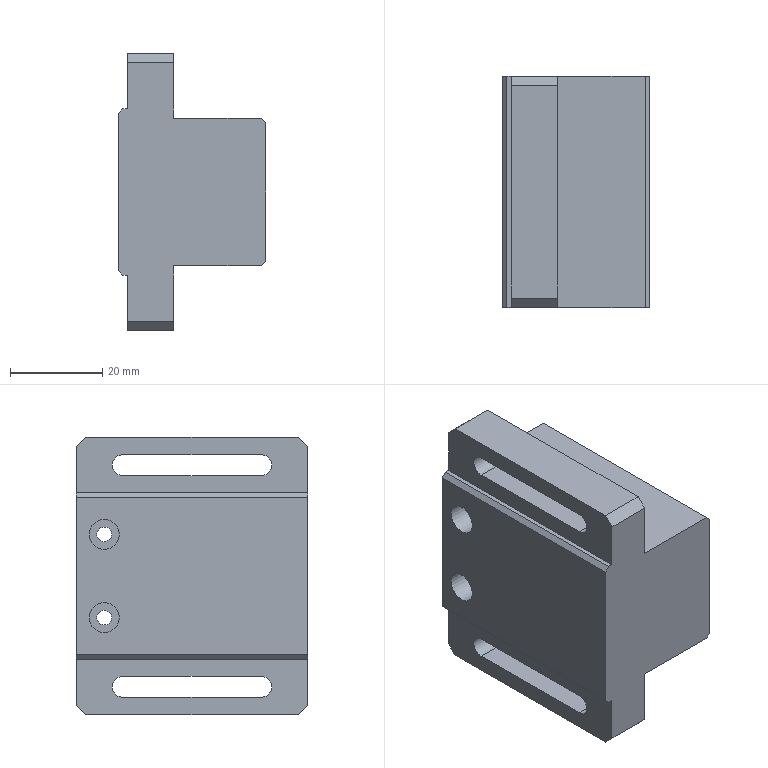Part | NX | 1 solid | 36 faces | box 32 x 50 x 60 mm | volume 61384 mm3 | plane 28 | cylinder 8 | commonest cylinder face diameters 4.5 x4 3.2 x2 6.5 x2
STEP:
#1=CARTESIAN_POINT('',(-15.,23.,-30.));
#2=VERTEX_POINT('',#1);
#3=CARTESIAN_POINT('',(-15.,-23.,-30.));
#4=VERTEX_POINT('',#3);
#5=CARTESIAN_POINT('',(-15.,25.,-30.));
#6=DIRECTION('',(0.,-1.,0.));
#7=VECTOR('',#6,1000.);
#8=LINE('',#5,#7);
#9=EDGE_CURVE('',#2,#4,#8,.T.);
#10=ORIENTED_EDGE('',*,*,#9,.F.);
#11=CARTESIAN_POINT('',(-5.,23.,-30.));
#12=VERTEX_POINT('',#11);
#13=CARTESIAN_POINT('',(-5.,23.,-30.));
#14=DIRECTION('',(1.,0.,0.));
#15=VECTOR('',#14,1000.);
#16=LINE('',#13,#15);
#17=EDGE_CURVE('',#2,#12,#16,.T.);
#18=ORIENTED_EDGE('',*,*,#17,.T.);
#19=CARTESIAN_POINT('',(-5.,-23.,-30.));
#20=VERTEX_POINT('',#19);
#21=CARTESIAN_POINT('',(-5.,25.,-30.));
#22=DIRECTION('',(0.,1.,0.));
#23=VECTOR('',#22,1000.);
#24=LINE('',#21,#23);
#25=EDGE_CURVE('',#20,#12,#24,.T.);
#26=ORIENTED_EDGE('',*,*,#25,.F.);
#27=CARTESIAN_POINT('',(-15.,-23.,-30.));
#28=DIRECTION('',(-1.,0.,0.));
#29=VECTOR('',#28,1000.);
#30=LINE('',#27,#29);
#31=EDGE_CURVE('',#20,#4,#30,.T.);
#32=ORIENTED_EDGE('',*,*,#31,.T.);
#33=EDGE_LOOP('',(#10,#18,#26,#32));
#34=FACE_BOUND('',#33,.T.);
#35=CARTESIAN_POINT('',(-15.,25.,-30.));
#36=DIRECTION('',(0.,0.,1.));
#37=DIRECTION('',(1.,0.,0.));
#38=AXIS2_PLACEMENT_3D('',#35,#36,#37);
#39=PLANE('',#38);
#40=ADVANCED_FACE('',(#34),#39,.F.);
#41=CARTESIAN_POINT('',(-15.,23.,30.));
#42=VERTEX_POINT('',#41);
#43=CARTESIAN_POINT('',(-15.,-23.,30.));
#44=VERTEX_POINT('',#43);
#45=CARTESIAN_POINT('',(-15.,25.,30.));
#46=DIRECTION('',(0.,-1.,0.));
#47=VECTOR('',#46,1000.);
#48=LINE('',#45,#47);
#49=EDGE_CURVE('',#42,#44,#48,.T.);
#50=ORIENTED_EDGE('',*,*,#49,.T.);
#51=CARTESIAN_POINT('',(-5.,-23.,30.));
#52=VERTEX_POINT('',#51);
#53=CARTESIAN_POINT('',(-15.,-23.,30.));
#54=DIRECTION('',(1.,0.,0.));
#55=VECTOR('',#54,1000.);
#56=LINE('',#53,#55);
#57=EDGE_CURVE('',#44,#52,#56,.T.);
#58=ORIENTED_EDGE('',*,*,#57,.T.);
#59=CARTESIAN_POINT('',(-5.,23.,30.));
#60=VERTEX_POINT('',#59);
#61=CARTESIAN_POINT('',(-5.,25.,30.));
#62=DIRECTION('',(0.,-1.,0.));
#63=VECTOR('',#62,1000.);
#64=LINE('',#61,#63);
#65=EDGE_CURVE('',#60,#52,#64,.T.);
#66=ORIENTED_EDGE('',*,*,#65,.F.);
#67=CARTESIAN_POINT('',(-15.,23.,30.));
#68=DIRECTION('',(-1.,0.,0.));
#69=VECTOR('',#68,1000.);
#70=LINE('',#67,#69);
#71=EDGE_CURVE('',#60,#42,#70,.T.);
#72=ORIENTED_EDGE('',*,*,#71,.T.);
#73=EDGE_LOOP('',(#50,#58,#66,#72));
#74=FACE_BOUND('',#73,.T.);
#75=CARTESIAN_POINT('',(-15.,25.,30.));
#76=DIRECTION('',(0.,0.,-1.));
#77=DIRECTION('',(-1.,0.,0.));
#78=AXIS2_PLACEMENT_3D('',#75,#76,#77);
#79=PLANE('',#78);
#80=ADVANCED_FACE('',(#74),#79,.F.);
#81=CARTESIAN_POINT('',(-5.,15.,-21.75));
#82=VERTEX_POINT('',#81);
#83=CARTESIAN_POINT('',(-5.,15.,-26.25));
#84=VERTEX_POINT('',#83);
#85=CARTESIAN_POINT('',(-5.,15.,-24.));
#86=DIRECTION('',(1.,0.,0.));
#87=DIRECTION('',(0.,0.,-1.));
#88=AXIS2_PLACEMENT_3D('',#85,#86,#87);
#89=CIRCLE('',#88,2.25);
#90=EDGE_CURVE('',#82,#84,#89,.F.);
#91=ORIENTED_EDGE('',*,*,#90,.F.);
#92=CARTESIAN_POINT('',(-15.,15.,-21.75));
#93=VERTEX_POINT('',#92);
#94=CARTESIAN_POINT('',(-17.,15.,-21.75));
#95=DIRECTION('',(1.,0.,0.));
#96=VECTOR('',#95,1000.);
#97=LINE('',#94,#96);
#98=EDGE_CURVE('',#93,#82,#97,.T.);
#99=ORIENTED_EDGE('',*,*,#98,.F.);
#100=CARTESIAN_POINT('',(-15.,15.,-26.25));
#101=VERTEX_POINT('',#100);
#102=CARTESIAN_POINT('',(-15.,15.,-24.));
#103=DIRECTION('',(1.,0.,0.));
#104=DIRECTION('',(0.,0.,-1.));
#105=AXIS2_PLACEMENT_3D('',#102,#103,#104);
#106=CIRCLE('',#105,2.25);
#107=EDGE_CURVE('',#101,#93,#106,.T.);
#108=ORIENTED_EDGE('',*,*,#107,.F.);
#109=CARTESIAN_POINT('',(-17.,15.,-26.25));
#110=DIRECTION('',(1.,0.,0.));
#111=VECTOR('',#110,1000.);
#112=LINE('',#109,#111);
#113=EDGE_CURVE('',#101,#84,#112,.T.);
#114=ORIENTED_EDGE('',*,*,#113,.T.);
#115=EDGE_LOOP('',(#91,#99,#108,#114));
#116=FACE_BOUND('',#115,.T.);
#117=CARTESIAN_POINT('',(-17.,15.,-24.));
#118=DIRECTION('',(1.,0.,0.));
#119=DIRECTION('',(0.,0.,-1.));
#120=AXIS2_PLACEMENT_3D('',#117,#118,#119);
#121=CYLINDRICAL_SURFACE('',#120,2.25);
#122=ADVANCED_FACE('',(#116),#121,.F.);
#123=CARTESIAN_POINT('',(-5.,-15.,-26.25));
#124=VERTEX_POINT('',#123);
#125=CARTESIAN_POINT('',(-5.,15.,-26.25));
#126=DIRECTION('',(0.,-1.,0.));
#127=VECTOR('',#126,1000.);
#128=LINE('',#125,#127);
#129=EDGE_CURVE('',#84,#124,#128,.T.);
#130=ORIENTED_EDGE('',*,*,#129,.F.);
#131=ORIENTED_EDGE('',*,*,#113,.F.);
#132=CARTESIAN_POINT('',(-15.,-15.,-26.25));
#133=VERTEX_POINT('',#132);
#134=CARTESIAN_POINT('',(-15.,25.,-26.25));
#135=DIRECTION('',(0.,1.,0.));
#136=VECTOR('',#135,1000.);
#137=LINE('',#134,#136);
#138=EDGE_CURVE('',#133,#101,#137,.T.);
#139=ORIENTED_EDGE('',*,*,#138,.F.);
#140=CARTESIAN_POINT('',(-17.,-15.,-26.25));
#141=DIRECTION('',(1.,0.,0.));
#142=VECTOR('',#141,1000.);
#143=LINE('',#140,#142);
#144=EDGE_CURVE('',#133,#124,#143,.T.);
#145=ORIENTED_EDGE('',*,*,#144,.T.);
#146=EDGE_LOOP('',(#130,#131,#139,#145));
#147=FACE_BOUND('',#146,.T.);
#148=CARTESIAN_POINT('',(-17.,15.,-26.25));
#149=DIRECTION('',(0.,0.,-1.));
#150=DIRECTION('',(-1.,0.,0.));
#151=AXIS2_PLACEMENT_3D('',#148,#149,#150);
#152=PLANE('',#151);
#153=ADVANCED_FACE('',(#147),#152,.F.);
#154=CARTESIAN_POINT('',(-5.,-15.,-21.75));
#155=VERTEX_POINT('',#154);
#156=CARTESIAN_POINT('',(-5.,-15.,-24.));
#157=DIRECTION('',(1.,0.,0.));
#158=DIRECTION('',(0.,0.,-1.));
#159=AXIS2_PLACEMENT_3D('',#156,#157,#158);
#160=CIRCLE('',#159,2.25);
#161=EDGE_CURVE('',#124,#155,#160,.F.);
#162=ORIENTED_EDGE('',*,*,#161,.F.);
#163=ORIENTED_EDGE('',*,*,#144,.F.);
#164=CARTESIAN_POINT('',(-15.,-15.,-21.75));
#165=VERTEX_POINT('',#164);
#166=CARTESIAN_POINT('',(-15.,-15.,-24.));
#167=DIRECTION('',(1.,0.,0.));
#168=DIRECTION('',(0.,0.,-1.));
#169=AXIS2_PLACEMENT_3D('',#166,#167,#168);
#170=CIRCLE('',#169,2.25);
#171=EDGE_CURVE('',#165,#133,#170,.T.);
#172=ORIENTED_EDGE('',*,*,#171,.F.);
#173=CARTESIAN_POINT('',(-17.,-15.,-21.75));
#174=DIRECTION('',(1.,0.,0.));
#175=VECTOR('',#174,1000.);
#176=LINE('',#173,#175);
#177=EDGE_CURVE('',#165,#155,#176,.T.);
#178=ORIENTED_EDGE('',*,*,#177,.T.);
#179=EDGE_LOOP('',(#162,#163,#172,#178));
#180=FACE_BOUND('',#179,.T.);
#181=CARTESIAN_POINT('',(-17.,-15.,-24.));
#182=DIRECTION('',(1.,0.,0.));
#183=DIRECTION('',(0.,0.,-1.));
#184=AXIS2_PLACEMENT_3D('',#181,#182,#183);
#185=CYLINDRICAL_SURFACE('',#184,2.25);
#186=ADVANCED_FACE('',(#180),#185,.F.);
#187=CARTESIAN_POINT('',(-5.,15.,-21.75));
#188=DIRECTION('',(0.,1.,0.));
#189=VECTOR('',#188,1000.);
#190=LINE('',#187,#189);
#191=EDGE_CURVE('',#155,#82,#190,.T.);
#192=ORIENTED_EDGE('',*,*,#191,.F.);
#193=ORIENTED_EDGE('',*,*,#177,.F.);
#194=CARTESIAN_POINT('',(-15.,25.,-21.75));
#195=DIRECTION('',(0.,-1.,0.));
#196=VECTOR('',#195,1000.);
#197=LINE('',#194,#196);
#198=EDGE_CURVE('',#93,#165,#197,.T.);
#199=ORIENTED_EDGE('',*,*,#198,.F.);
#200=ORIENTED_EDGE('',*,*,#98,.T.);
#201=EDGE_LOOP('',(#192,#193,#199,#200));
#202=FACE_BOUND('',#201,.T.);
#203=CARTESIAN_POINT('',(-17.,15.,-21.75));
#204=DIRECTION('',(0.,0.,1.));
#205=DIRECTION('',(1.,0.,0.));
#206=AXIS2_PLACEMENT_3D('',#203,#204,#205);
#207=PLANE('',#206);
#208=ADVANCED_FACE('',(#202),#207,.F.);
#209=CARTESIAN_POINT('',(-5.,15.,26.25));
#210=VERTEX_POINT('',#209);
#211=CARTESIAN_POINT('',(-5.,15.,21.75));
#212=VERTEX_POINT('',#211);
#213=CARTESIAN_POINT('',(-5.,15.,24.));
#214=DIRECTION('',(1.,0.,0.));
#215=DIRECTION('',(0.,0.,-1.));
#216=AXIS2_PLACEMENT_3D('',#213,#214,#215);
#217=CIRCLE('',#216,2.25);
#218=EDGE_CURVE('',#210,#212,#217,.F.);
#219=ORIENTED_EDGE('',*,*,#218,.F.);
#220=CARTESIAN_POINT('',(-15.,15.,26.25));
#221=VERTEX_POINT('',#220);
#222=CARTESIAN_POINT('',(-17.,15.,26.25));
#223=DIRECTION('',(1.,0.,0.));
#224=VECTOR('',#223,1000.);
#225=LINE('',#222,#224);
#226=EDGE_CURVE('',#221,#210,#225,.T.);
#227=ORIENTED_EDGE('',*,*,#226,.F.);
#228=CARTESIAN_POINT('',(-15.,15.,21.75));
#229=VERTEX_POINT('',#228);
#230=CARTESIAN_POINT('',(-15.,15.,24.));
#231=DIRECTION('',(1.,0.,0.));
#232=DIRECTION('',(0.,0.,-1.));
#233=AXIS2_PLACEMENT_3D('',#230,#231,#232);
#234=CIRCLE('',#233,2.25);
#235=EDGE_CURVE('',#229,#221,#234,.T.);
#236=ORIENTED_EDGE('',*,*,#235,.F.);
#237=CARTESIAN_POINT('',(-17.,15.,21.75));
#238=DIRECTION('',(1.,0.,0.));
#239=VECTOR('',#238,1000.);
#240=LINE('',#237,#239);
#241=EDGE_CURVE('',#229,#212,#240,.T.);
#242=ORIENTED_EDGE('',*,*,#241,.T.);
#243=EDGE_LOOP('',(#219,#227,#236,#242));
#244=FACE_BOUND('',#243,.T.);
#245=CARTESIAN_POINT('',(-17.,15.,24.));
#246=DIRECTION('',(1.,0.,0.));
#247=DIRECTION('',(0.,0.,-1.));
#248=AXIS2_PLACEMENT_3D('',#245,#246,#247);
#249=CYLINDRICAL_SURFACE('',#248,2.25);
#250=ADVANCED_FACE('',(#244),#249,.F.);
#251=CARTESIAN_POINT('',(-5.,-15.,21.75));
#252=VERTEX_POINT('',#251);
#253=CARTESIAN_POINT('',(-5.,15.,21.75));
#254=DIRECTION('',(0.,-1.,0.));
#255=VECTOR('',#254,1000.);
#256=LINE('',#253,#255);
#257=EDGE_CURVE('',#212,#252,#256,.T.);
#258=ORIENTED_EDGE('',*,*,#257,.F.);
#259=ORIENTED_EDGE('',*,*,#241,.F.);
#260=CARTESIAN_POINT('',(-15.,-15.,21.75));
#261=VERTEX_POINT('',#260);
#262=CARTESIAN_POINT('',(-15.,25.,21.75));
#263=DIRECTION('',(0.,1.,0.));
#264=VECTOR('',#263,1000.);
#265=LINE('',#262,#264);
#266=EDGE_CURVE('',#261,#229,#265,.T.);
#267=ORIENTED_EDGE('',*,*,#266,.F.);
#268=CARTESIAN_POINT('',(-17.,-15.,21.75));
#269=DIRECTION('',(1.,0.,0.));
#270=VECTOR('',#269,1000.);
#271=LINE('',#268,#270);
#272=EDGE_CURVE('',#261,#252,#271,.T.);
#273=ORIENTED_EDGE('',*,*,#272,.T.);
#274=EDGE_LOOP('',(#258,#259,#267,#273));
#275=FACE_BOUND('',#274,.T.);
#276=CARTESIAN_POINT('',(-17.,15.,21.75));
#277=DIRECTION('',(0.,0.,-1.));
#278=DIRECTION('',(-1.,0.,0.));
#279=AXIS2_PLACEMENT_3D('',#276,#277,#278);
#280=PLANE('',#279);
#281=ADVANCED_FACE('',(#275),#280,.F.);
#282=CARTESIAN_POINT('',(-5.,-15.,26.25));
#283=VERTEX_POINT('',#282);
#284=CARTESIAN_POINT('',(-5.,-15.,24.));
#285=DIRECTION('',(1.,0.,0.));
#286=DIRECTION('',(0.,0.,-1.));
#287=AXIS2_PLACEMENT_3D('',#284,#285,#286);
#288=CIRCLE('',#287,2.25);
#289=EDGE_CURVE('',#252,#283,#288,.F.);
#290=ORIENTED_EDGE('',*,*,#289,.F.);
#291=ORIENTED_EDGE('',*,*,#272,.F.);
#292=CARTESIAN_POINT('',(-15.,-15.,26.25));
#293=VERTEX_POINT('',#292);
#294=CARTESIAN_POINT('',(-15.,-15.,24.));
#295=DIRECTION('',(1.,0.,0.));
#296=DIRECTION('',(0.,0.,-1.));
#297=AXIS2_PLACEMENT_3D('',#294,#295,#296);
#298=CIRCLE('',#297,2.25);
#299=EDGE_CURVE('',#293,#261,#298,.T.);
#300=ORIENTED_EDGE('',*,*,#299,.F.);
#301=CARTESIAN_POINT('',(-17.,-15.,26.25));
#302=DIRECTION('',(1.,0.,0.));
#303=VECTOR('',#302,1000.);
#304=LINE('',#301,#303);
#305=EDGE_CURVE('',#293,#283,#304,.T.);
#306=ORIENTED_EDGE('',*,*,#305,.T.);
#307=EDGE_LOOP('',(#290,#291,#300,#306));
#308=FACE_BOUND('',#307,.T.);
#309=CARTESIAN_POINT('',(-17.,-15.,24.));
#310=DIRECTION('',(1.,0.,0.));
#311=DIRECTION('',(0.,0.,-1.));
#312=AXIS2_PLACEMENT_3D('',#309,#310,#311);
#313=CYLINDRICAL_SURFACE('',#312,2.25);
#314=ADVANCED_FACE('',(#308),#313,.F.);
#315=CARTESIAN_POINT('',(-5.,15.,26.25));
#316=DIRECTION('',(0.,1.,0.));
#317=VECTOR('',#316,1000.);
#318=LINE('',#315,#317);
#319=EDGE_CURVE('',#283,#210,#318,.T.);
#320=ORIENTED_EDGE('',*,*,#319,.F.);
#321=ORIENTED_EDGE('',*,*,#305,.F.);
#322=CARTESIAN_POINT('',(-15.,25.,26.25));
#323=DIRECTION('',(0.,-1.,0.));
#324=VECTOR('',#323,1000.);
#325=LINE('',#322,#324);
#326=EDGE_CURVE('',#221,#293,#325,.T.);
#327=ORIENTED_EDGE('',*,*,#326,.F.);
#328=ORIENTED_EDGE('',*,*,#226,.T.);
#329=EDGE_LOOP('',(#320,#321,#327,#328));
#330=FACE_BOUND('',#329,.T.);
#331=CARTESIAN_POINT('',(-17.,15.,26.25));
#332=DIRECTION('',(0.,0.,1.));
#333=DIRECTION('',(1.,0.,0.));
#334=AXIS2_PLACEMENT_3D('',#331,#332,#333);
#335=PLANE('',#334);
#336=ADVANCED_FACE('',(#330),#335,.F.);
#337=ORIENTED_EDGE('',*,*,#138,.T.);
#338=ORIENTED_EDGE('',*,*,#107,.T.);
#339=ORIENTED_EDGE('',*,*,#198,.T.);
#340=ORIENTED_EDGE('',*,*,#171,.T.);
#341=EDGE_LOOP('',(#337,#338,#339,#340));
#342=FACE_BOUND('',#341,.T.);
#343=CARTESIAN_POINT('',(-15.,25.,-28.));
#344=VERTEX_POINT('',#343);
#345=CARTESIAN_POINT('',(-15.,25.,-18.));
#346=VERTEX_POINT('',#345);
#347=CARTESIAN_POINT('',(-15.,25.,-30.));
#348=DIRECTION('',(0.,0.,1.));
#349=VECTOR('',#348,1000.);
#350=LINE('',#347,#349);
#351=EDGE_CURVE('',#344,#346,#350,.T.);
#352=ORIENTED_EDGE('',*,*,#351,.F.);
#353=CARTESIAN_POINT('',(-15.,25.,-28.));
#354=DIRECTION('',(0.,-0.7071,-0.7071));
#355=VECTOR('',#354,1000.);
#356=LINE('',#353,#355);
#357=EDGE_CURVE('',#344,#2,#356,.T.);
#358=ORIENTED_EDGE('',*,*,#357,.T.);
#359=ORIENTED_EDGE('',*,*,#9,.T.);
#360=CARTESIAN_POINT('',(-15.,-25.,-28.));
#361=VERTEX_POINT('',#360);
#362=CARTESIAN_POINT('',(-15.,-23.,-30.));
#363=DIRECTION('',(0.,0.7071,-0.7071));
#364=VECTOR('',#363,1000.);
#365=LINE('',#362,#364);
#366=EDGE_CURVE('',#4,#361,#365,.F.);
#367=ORIENTED_EDGE('',*,*,#366,.T.);
#368=CARTESIAN_POINT('',(-15.,-25.,-18.));
#369=VERTEX_POINT('',#368);
#370=CARTESIAN_POINT('',(-15.,-25.,-30.));
#371=DIRECTION('',(0.,0.,1.));
#372=VECTOR('',#371,1000.);
#373=LINE('',#370,#372);
#374=EDGE_CURVE('',#361,#369,#373,.T.);
#375=ORIENTED_EDGE('',*,*,#374,.T.);
#376=CARTESIAN_POINT('',(-15.,-25.,-18.));
#377=DIRECTION('',(0.,1.,0.));
#378=VECTOR('',#377,1000.);
#379=LINE('',#376,#378);
#380=EDGE_CURVE('',#369,#346,#379,.T.);
#381=ORIENTED_EDGE('',*,*,#380,.T.);
#382=EDGE_LOOP('',(#352,#358,#359,#367,#375,#381));
#383=FACE_BOUND('',#382,.T.);
#384=CARTESIAN_POINT('',(-15.,25.,-30.));
#385=DIRECTION('',(1.,0.,0.));
#386=DIRECTION('',(0.,0.,-1.));
#387=AXIS2_PLACEMENT_3D('',#384,#385,#386);
#388=PLANE('',#387);
#389=ADVANCED_FACE('',(#342,#383),#388,.F.);
#390=CARTESIAN_POINT('',(15.,19.,-7.4));
#391=VERTEX_POINT('',#390);
#392=CARTESIAN_POINT('',(15.,19.,-9.));
#393=DIRECTION('',(-1.,0.,0.));
#394=DIRECTION('',(0.,0.,1.));
#395=AXIS2_PLACEMENT_3D('',#392,#393,#394);
#396=CIRCLE('',#395,1.6);
#397=EDGE_CURVE('',#391,#391,#396,.T.);
#398=ORIENTED_EDGE('',*,*,#397,.T.);
#399=EDGE_LOOP('',(#398));
#400=FACE_BOUND('',#399,.T.);
#401=CARTESIAN_POINT('',(15.,19.,10.6));
#402=VERTEX_POINT('',#401);
#403=CARTESIAN_POINT('',(15.,19.,9.));
#404=DIRECTION('',(-1.,0.,0.));
#405=DIRECTION('',(0.,0.,1.));
#406=AXIS2_PLACEMENT_3D('',#403,#404,#405);
#407=CIRCLE('',#406,1.6);
#408=EDGE_CURVE('',#402,#402,#407,.T.);
#409=ORIENTED_EDGE('',*,*,#408,.T.);
#410=EDGE_LOOP('',(#409));
#411=FACE_BOUND('',#410,.T.);
#412=CARTESIAN_POINT('',(15.,25.,15.));
#413=VERTEX_POINT('',#412);
#414=CARTESIAN_POINT('',(15.,25.,-15.));
#415=VERTEX_POINT('',#414);
#416=CARTESIAN_POINT('',(15.,25.,-30.));
#417=DIRECTION('',(0.,0.,-1.));
#418=VECTOR('',#417,1000.);
#419=LINE('',#416,#418);
#420=EDGE_CURVE('',#413,#415,#419,.T.);
#421=ORIENTED_EDGE('',*,*,#420,.F.);
#422=CARTESIAN_POINT('',(15.,-25.,15.));
#423=VERTEX_POINT('',#422);
#424=CARTESIAN_POINT('',(15.,25.,15.));
#425=DIRECTION('',(0.,-1.,0.));
#426=VECTOR('',#425,1000.);
#427=LINE('',#424,#426);
#428=EDGE_CURVE('',#413,#423,#427,.T.);
#429=ORIENTED_EDGE('',*,*,#428,.T.);
#430=CARTESIAN_POINT('',(15.,-25.,-15.));
#431=VERTEX_POINT('',#430);
#432=CARTESIAN_POINT('',(15.,-25.,-30.));
#433=DIRECTION('',(0.,0.,-1.));
#434=VECTOR('',#433,1000.);
#435=LINE('',#432,#434);
#436=EDGE_CURVE('',#423,#431,#435,.T.);
#437=ORIENTED_EDGE('',*,*,#436,.T.);
#438=CARTESIAN_POINT('',(15.,25.,-15.));
#439=DIRECTION('',(0.,1.,0.));
#440=VECTOR('',#439,1000.);
#441=LINE('',#438,#440);
#442=EDGE_CURVE('',#431,#415,#441,.T.);
#443=ORIENTED_EDGE('',*,*,#442,.T.);
#444=EDGE_LOOP('',(#421,#429,#437,#443));
#445=FACE_BOUND('',#444,.T.);
#446=CARTESIAN_POINT('',(15.,25.,-30.));
#447=DIRECTION('',(-1.,0.,0.));
#448=DIRECTION('',(0.,0.,1.));
#449=AXIS2_PLACEMENT_3D('',#446,#447,#448);
#450=PLANE('',#449);
#451=ADVANCED_FACE('',(#400,#411,#445),#450,.F.);
#452=ORIENTED_EDGE('',*,*,#266,.T.);
#453=ORIENTED_EDGE('',*,*,#235,.T.);
#454=ORIENTED_EDGE('',*,*,#326,.T.);
#455=ORIENTED_EDGE('',*,*,#299,.T.);
#456=EDGE_LOOP('',(#452,#453,#454,#455));
#457=FACE_BOUND('',#456,.T.);
#458=CARTESIAN_POINT('',(-15.,-25.,18.));
#459=VERTEX_POINT('',#458);
#460=CARTESIAN_POINT('',(-15.,-25.,28.));
#461=VERTEX_POINT('',#460);
#462=CARTESIAN_POINT('',(-15.,-25.,-30.));
#463=DIRECTION('',(0.,0.,1.));
#464=VECTOR('',#463,1000.);
#465=LINE('',#462,#464);
#466=EDGE_CURVE('',#459,#461,#465,.T.);
#467=ORIENTED_EDGE('',*,*,#466,.T.);
#468=CARTESIAN_POINT('',(-15.,-23.,30.));
#469=DIRECTION('',(0.,-0.7071,-0.7071));
#470=VECTOR('',#469,1000.);
#471=LINE('',#468,#470);
#472=EDGE_CURVE('',#461,#44,#471,.F.);
#473=ORIENTED_EDGE('',*,*,#472,.T.);
#474=ORIENTED_EDGE('',*,*,#49,.F.);
#475=CARTESIAN_POINT('',(-15.,25.,28.));
#476=VERTEX_POINT('',#475);
#477=CARTESIAN_POINT('',(-15.,25.,28.));
#478=DIRECTION('',(0.,0.7071,-0.7071));
#479=VECTOR('',#478,1000.);
#480=LINE('',#477,#479);
#481=EDGE_CURVE('',#42,#476,#480,.T.);
#482=ORIENTED_EDGE('',*,*,#481,.T.);
#483=CARTESIAN_POINT('',(-15.,25.,18.));
#484=VERTEX_POINT('',#483);
#485=CARTESIAN_POINT('',(-15.,25.,-30.));
#486=DIRECTION('',(0.,0.,1.));
#487=VECTOR('',#486,1000.);
#488=LINE('',#485,#487);
#489=EDGE_CURVE('',#484,#476,#488,.T.);
#490=ORIENTED_EDGE('',*,*,#489,.F.);
#491=CARTESIAN_POINT('',(-15.,-25.,18.));
#492=DIRECTION('',(0.,-1.,0.));
#493=VECTOR('',#492,1000.);
#494=LINE('',#491,#493);
#495=EDGE_CURVE('',#484,#459,#494,.T.);
#496=ORIENTED_EDGE('',*,*,#495,.T.);
#497=EDGE_LOOP('',(#467,#473,#474,#482,#490,#496));
#498=FACE_BOUND('',#497,.T.);
#499=CARTESIAN_POINT('',(-15.,25.,-30.));
#500=DIRECTION('',(1.,0.,0.));
#501=DIRECTION('',(0.,0.,-1.));
#502=AXIS2_PLACEMENT_3D('',#499,#500,#501);
#503=PLANE('',#502);
#504=ADVANCED_FACE('',(#457,#498),#503,.F.);
#505=CARTESIAN_POINT('',(-5.,25.,16.));
#506=VERTEX_POINT('',#505);
#507=CARTESIAN_POINT('',(14.,25.,16.));
#508=VERTEX_POINT('',#507);
#509=CARTESIAN_POINT('',(-5.,25.,16.));
#510=DIRECTION('',(1.,0.,0.));
#511=VECTOR('',#510,1000.);
#512=LINE('',#509,#511);
#513=EDGE_CURVE('',#506,#508,#512,.T.);
#514=ORIENTED_EDGE('',*,*,#513,.T.);
#515=CARTESIAN_POINT('',(15.,25.,15.));
#516=DIRECTION('',(-0.7071,0.,0.7071));
#517=VECTOR('',#516,1000.);
#518=LINE('',#515,#517);
#519=EDGE_CURVE('',#508,#413,#518,.F.);
#520=ORIENTED_EDGE('',*,*,#519,.T.);
#521=ORIENTED_EDGE('',*,*,#420,.T.);
#522=CARTESIAN_POINT('',(14.,25.,-16.));
#523=VERTEX_POINT('',#522);
#524=CARTESIAN_POINT('',(15.,25.,-15.));
#525=DIRECTION('',(0.7071,0.,0.7071));
#526=VECTOR('',#525,1000.);
#527=LINE('',#524,#526);
#528=EDGE_CURVE('',#415,#523,#527,.F.);
#529=ORIENTED_EDGE('',*,*,#528,.T.);
#530=CARTESIAN_POINT('',(-5.,25.,-16.));
#531=VERTEX_POINT('',#530);
#532=CARTESIAN_POINT('',(-5.,25.,-16.));
#533=DIRECTION('',(1.,0.,0.));
#534=VECTOR('',#533,1000.);
#535=LINE('',#532,#534);
#536=EDGE_CURVE('',#531,#523,#535,.T.);
#537=ORIENTED_EDGE('',*,*,#536,.F.);
#538=CARTESIAN_POINT('',(-5.,25.,-28.));
#539=VERTEX_POINT('',#538);
#540=CARTESIAN_POINT('',(-5.,25.,-16.));
#541=DIRECTION('',(0.,0.,1.));
#542=VECTOR('',#541,1000.);
#543=LINE('',#540,#542);
#544=EDGE_CURVE('',#539,#531,#543,.T.);
#545=ORIENTED_EDGE('',*,*,#544,.F.);
#546=CARTESIAN_POINT('',(-15.,25.,-28.));
#547=DIRECTION('',(-1.,0.,0.));
#548=VECTOR('',#547,1000.);
#549=LINE('',#546,#548);
#550=EDGE_CURVE('',#539,#344,#549,.T.);
#551=ORIENTED_EDGE('',*,*,#550,.T.);
#552=ORIENTED_EDGE('',*,*,#351,.T.);
#553=CARTESIAN_POINT('',(-16.,25.,-18.));
#554=VERTEX_POINT('',#553);
#555=CARTESIAN_POINT('',(-17.,25.,-18.));
#556=DIRECTION('',(1.,0.,0.));
#557=VECTOR('',#556,1000.);
#558=LINE('',#555,#557);
#559=EDGE_CURVE('',#554,#346,#558,.T.);
#560=ORIENTED_EDGE('',*,*,#559,.F.);
#561=CARTESIAN_POINT('',(-17.,25.,-17.));
#562=VERTEX_POINT('',#561);
#563=CARTESIAN_POINT('',(-17.,25.,-17.));
#564=DIRECTION('',(0.7071,0.,-0.7071));
#565=VECTOR('',#564,1000.);
#566=LINE('',#563,#565);
#567=EDGE_CURVE('',#554,#562,#566,.F.);
#568=ORIENTED_EDGE('',*,*,#567,.T.);
#569=CARTESIAN_POINT('',(-17.,25.,17.));
#570=VERTEX_POINT('',#569);
#571=CARTESIAN_POINT('',(-17.,25.,18.));
#572=DIRECTION('',(0.,0.,1.));
#573=VECTOR('',#572,1000.);
#574=LINE('',#571,#573);
#575=EDGE_CURVE('',#562,#570,#574,.T.);
#576=ORIENTED_EDGE('',*,*,#575,.T.);
#577=CARTESIAN_POINT('',(-16.,25.,18.));
#578=VERTEX_POINT('',#577);
#579=CARTESIAN_POINT('',(-17.,25.,17.));
#580=DIRECTION('',(-0.7071,0.,-0.7071));
#581=VECTOR('',#580,1000.);
#582=LINE('',#579,#581);
#583=EDGE_CURVE('',#570,#578,#582,.F.);
#584=ORIENTED_EDGE('',*,*,#583,.T.);
#585=CARTESIAN_POINT('',(-17.,25.,18.));
#586=DIRECTION('',(1.,0.,0.));
#587=VECTOR('',#586,1000.);
#588=LINE('',#585,#587);
#589=EDGE_CURVE('',#578,#484,#588,.T.);
#590=ORIENTED_EDGE('',*,*,#589,.T.);
#591=ORIENTED_EDGE('',*,*,#489,.T.);
#592=CARTESIAN_POINT('',(-5.,25.,28.));
#593=VERTEX_POINT('',#592);
#594=CARTESIAN_POINT('',(-5.,25.,28.));
#595=DIRECTION('',(1.,0.,0.));
#596=VECTOR('',#595,1000.);
#597=LINE('',#594,#596);
#598=EDGE_CURVE('',#476,#593,#597,.T.);
#599=ORIENTED_EDGE('',*,*,#598,.T.);
#600=CARTESIAN_POINT('',(-5.,25.,30.));
#601=DIRECTION('',(0.,0.,1.));
#602=VECTOR('',#601,1000.);
#603=LINE('',#600,#602);
#604=EDGE_CURVE('',#506,#593,#603,.T.);
#605=ORIENTED_EDGE('',*,*,#604,.F.);
#606=EDGE_LOOP('',(#514,#520,#521,#529,#537,#545,#551,#552,#560,#568,#576,#584,#590,#591,#599,#605));
#607=FACE_BOUND('',#606,.T.);
#608=CARTESIAN_POINT('',(0.,25.,0.));
#609=DIRECTION('',(0.,1.,0.));
#610=DIRECTION('',(0.,0.,1.));
#611=AXIS2_PLACEMENT_3D('',#608,#609,#610);
#612=PLANE('',#611);
#613=ADVANCED_FACE('',(#607),#612,.T.);
#614=ORIENTED_EDGE('',*,*,#436,.F.);
#615=CARTESIAN_POINT('',(14.,-25.,16.));
#616=VERTEX_POINT('',#615);
#617=CARTESIAN_POINT('',(14.,-25.,16.));
#618=DIRECTION('',(0.7071,0.,-0.7071));
#619=VECTOR('',#618,1000.);
#620=LINE('',#617,#619);
#621=EDGE_CURVE('',#423,#616,#620,.F.);
#622=ORIENTED_EDGE('',*,*,#621,.T.);
#623=CARTESIAN_POINT('',(-5.,-25.,16.));
#624=VERTEX_POINT('',#623);
#625=CARTESIAN_POINT('',(-5.,-25.,16.));
#626=DIRECTION('',(1.,0.,0.));
#627=VECTOR('',#626,1000.);
#628=LINE('',#625,#627);
#629=EDGE_CURVE('',#624,#616,#628,.T.);
#630=ORIENTED_EDGE('',*,*,#629,.F.);
#631=CARTESIAN_POINT('',(-5.,-25.,28.));
#632=VERTEX_POINT('',#631);
#633=CARTESIAN_POINT('',(-5.,-25.,30.));
#634=DIRECTION('',(0.,0.,-1.));
#635=VECTOR('',#634,1000.);
#636=LINE('',#633,#635);
#637=EDGE_CURVE('',#632,#624,#636,.T.);
#638=ORIENTED_EDGE('',*,*,#637,.F.);
#639=CARTESIAN_POINT('',(0.,-25.,28.));
#640=DIRECTION('',(-1.,0.,0.));
#641=VECTOR('',#640,1000.);
#642=LINE('',#639,#641);
#643=EDGE_CURVE('',#632,#461,#642,.T.);
#644=ORIENTED_EDGE('',*,*,#643,.T.);
#645=ORIENTED_EDGE('',*,*,#466,.F.);
#646=CARTESIAN_POINT('',(-16.,-25.,18.));
#647=VERTEX_POINT('',#646);
#648=CARTESIAN_POINT('',(-17.,-25.,18.));
#649=DIRECTION('',(1.,0.,0.));
#650=VECTOR('',#649,1000.);
#651=LINE('',#648,#650);
#652=EDGE_CURVE('',#647,#459,#651,.T.);
#653=ORIENTED_EDGE('',*,*,#652,.F.);
#654=CARTESIAN_POINT('',(-17.,-25.,17.));
#655=VERTEX_POINT('',#654);
#656=CARTESIAN_POINT('',(-16.,-25.,18.));
#657=DIRECTION('',(0.7071,0.,0.7071));
#658=VECTOR('',#657,1000.);
#659=LINE('',#656,#658);
#660=EDGE_CURVE('',#647,#655,#659,.F.);
#661=ORIENTED_EDGE('',*,*,#660,.T.);
#662=CARTESIAN_POINT('',(-17.,-25.,-17.));
#663=VERTEX_POINT('',#662);
#664=CARTESIAN_POINT('',(-17.,-25.,18.));
#665=DIRECTION('',(0.,0.,-1.));
#666=VECTOR('',#665,1000.);
#667=LINE('',#664,#666);
#668=EDGE_CURVE('',#655,#663,#667,.T.);
#669=ORIENTED_EDGE('',*,*,#668,.T.);
#670=CARTESIAN_POINT('',(-16.,-25.,-18.));
#671=VERTEX_POINT('',#670);
#672=CARTESIAN_POINT('',(-16.,-25.,-18.));
#673=DIRECTION('',(-0.7071,0.,0.7071));
#674=VECTOR('',#673,1000.);
#675=LINE('',#672,#674);
#676=EDGE_CURVE('',#663,#671,#675,.F.);
#677=ORIENTED_EDGE('',*,*,#676,.T.);
#678=CARTESIAN_POINT('',(-17.,-25.,-18.));
#679=DIRECTION('',(1.,0.,0.));
#680=VECTOR('',#679,1000.);
#681=LINE('',#678,#680);
#682=EDGE_CURVE('',#671,#369,#681,.T.);
#683=ORIENTED_EDGE('',*,*,#682,.T.);
#684=ORIENTED_EDGE('',*,*,#374,.F.);
#685=CARTESIAN_POINT('',(-5.,-25.,-28.));
#686=VERTEX_POINT('',#685);
#687=CARTESIAN_POINT('',(0.,-25.,-28.));
#688=DIRECTION('',(1.,0.,0.));
#689=VECTOR('',#688,1000.);
#690=LINE('',#687,#689);
#691=EDGE_CURVE('',#361,#686,#690,.T.);
#692=ORIENTED_EDGE('',*,*,#691,.T.);
#693=CARTESIAN_POINT('',(-5.,-25.,-16.));
#694=VERTEX_POINT('',#693);
#695=CARTESIAN_POINT('',(-5.,-25.,-16.));
#696=DIRECTION('',(0.,0.,-1.));
#697=VECTOR('',#696,1000.);
#698=LINE('',#695,#697);
#699=EDGE_CURVE('',#694,#686,#698,.T.);
#700=ORIENTED_EDGE('',*,*,#699,.F.);
#701=CARTESIAN_POINT('',(14.,-25.,-16.));
#702=VERTEX_POINT('',#701);
#703=CARTESIAN_POINT('',(-5.,-25.,-16.));
#704=DIRECTION('',(1.,0.,0.));
#705=VECTOR('',#704,1000.);
#706=LINE('',#703,#705);
#707=EDGE_CURVE('',#694,#702,#706,.T.);
#708=ORIENTED_EDGE('',*,*,#707,.T.);
#709=CARTESIAN_POINT('',(14.,-25.,-16.));
#710=DIRECTION('',(-0.7071,0.,-0.7071));
#711=VECTOR('',#710,1000.);
#712=LINE('',#709,#711);
#713=EDGE_CURVE('',#702,#431,#712,.F.);
#714=ORIENTED_EDGE('',*,*,#713,.T.);
#715=EDGE_LOOP('',(#614,#622,#630,#638,#644,#645,#653,#661,#669,#677,#683,#684,#692,#700,#708,#714));
#716=FACE_BOUND('',#715,.T.);
#717=CARTESIAN_POINT('',(0.,-25.,0.));
#718=DIRECTION('',(0.,1.,0.));
#719=DIRECTION('',(0.,0.,1.));
#720=AXIS2_PLACEMENT_3D('',#717,#718,#719);
#721=PLANE('',#720);
#722=ADVANCED_FACE('',(#716),#721,.F.);
#723=ORIENTED_EDGE('',*,*,#682,.F.);
#724=CARTESIAN_POINT('',(-16.,-25.,-18.));
#725=DIRECTION('',(0.,1.,0.));
#726=VECTOR('',#725,1000.);
#727=LINE('',#724,#726);
#728=EDGE_CURVE('',#671,#554,#727,.T.);
#729=ORIENTED_EDGE('',*,*,#728,.T.);
#730=ORIENTED_EDGE('',*,*,#559,.T.);
#731=ORIENTED_EDGE('',*,*,#380,.F.);
#732=EDGE_LOOP('',(#723,#729,#730,#731));
#733=FACE_BOUND('',#732,.T.);
#734=CARTESIAN_POINT('',(-17.,-25.,-18.));
#735=DIRECTION('',(0.,0.,-1.));
#736=DIRECTION('',(-1.,0.,0.));
#737=AXIS2_PLACEMENT_3D('',#734,#735,#736);
#738=PLANE('',#737);
#739=ADVANCED_FACE('',(#733),#738,.T.);
#740=ORIENTED_EDGE('',*,*,#589,.F.);
#741=CARTESIAN_POINT('',(-16.,-25.,18.));
#742=DIRECTION('',(0.,-1.,0.));
#743=VECTOR('',#742,1000.);
#744=LINE('',#741,#743);
#745=EDGE_CURVE('',#578,#647,#744,.T.);
#746=ORIENTED_EDGE('',*,*,#745,.T.);
#747=ORIENTED_EDGE('',*,*,#652,.T.);
#748=ORIENTED_EDGE('',*,*,#495,.F.);
#749=EDGE_LOOP('',(#740,#746,#747,#748));
#750=FACE_BOUND('',#749,.T.);
#751=CARTESIAN_POINT('',(-17.,-25.,18.));
#752=DIRECTION('',(0.,0.,1.));
#753=DIRECTION('',(1.,0.,0.));
#754=AXIS2_PLACEMENT_3D('',#751,#752,#753);
#755=PLANE('',#754);
#756=ADVANCED_FACE('',(#750),#755,.T.);
#757=CARTESIAN_POINT('',(-17.,19.,-5.75));
#758=VERTEX_POINT('',#757);
#759=CARTESIAN_POINT('',(-17.,19.,-9.));
#760=DIRECTION('',(-1.,0.,0.));
#761=DIRECTION('',(0.,0.,1.));
#762=AXIS2_PLACEMENT_3D('',#759,#760,#761);
#763=CIRCLE('',#762,3.25);
#764=EDGE_CURVE('',#758,#758,#763,.T.);
#765=ORIENTED_EDGE('',*,*,#764,.F.);
#766=EDGE_LOOP('',(#765));
#767=FACE_BOUND('',#766,.T.);
#768=CARTESIAN_POINT('',(-17.,19.,12.25));
#769=VERTEX_POINT('',#768);
#770=CARTESIAN_POINT('',(-17.,19.,9.));
#771=DIRECTION('',(-1.,0.,0.));
#772=DIRECTION('',(0.,0.,1.));
#773=AXIS2_PLACEMENT_3D('',#770,#771,#772);
#774=CIRCLE('',#773,3.25);
#775=EDGE_CURVE('',#769,#769,#774,.T.);
#776=ORIENTED_EDGE('',*,*,#775,.F.);
#777=EDGE_LOOP('',(#776));
#778=FACE_BOUND('',#777,.T.);
#779=ORIENTED_EDGE('',*,*,#575,.F.);
#780=CARTESIAN_POINT('',(-17.,0.,-17.));
#781=DIRECTION('',(0.,-1.,0.));
#782=VECTOR('',#781,1000.);
#783=LINE('',#780,#782);
#784=EDGE_CURVE('',#562,#663,#783,.T.);
#785=ORIENTED_EDGE('',*,*,#784,.T.);
#786=ORIENTED_EDGE('',*,*,#668,.F.);
#787=CARTESIAN_POINT('',(-17.,0.,17.));
#788=DIRECTION('',(0.,1.,0.));
#789=VECTOR('',#788,1000.);
#790=LINE('',#787,#789);
#791=EDGE_CURVE('',#655,#570,#790,.T.);
#792=ORIENTED_EDGE('',*,*,#791,.T.);
#793=EDGE_LOOP('',(#779,#785,#786,#792));
#794=FACE_BOUND('',#793,.T.);
#795=CARTESIAN_POINT('',(-17.,0.,0.));
#796=DIRECTION('',(-1.,0.,0.));
#797=DIRECTION('',(0.,0.,1.));
#798=AXIS2_PLACEMENT_3D('',#795,#796,#797);
#799=PLANE('',#798);
#800=ADVANCED_FACE('',(#767,#778,#794),#799,.T.);
#801=ORIENTED_EDGE('',*,*,#218,.T.);
#802=ORIENTED_EDGE('',*,*,#257,.T.);
#803=ORIENTED_EDGE('',*,*,#289,.T.);
#804=ORIENTED_EDGE('',*,*,#319,.T.);
#805=EDGE_LOOP('',(#801,#802,#803,#804));
#806=FACE_BOUND('',#805,.T.);
#807=ORIENTED_EDGE('',*,*,#65,.T.);
#808=CARTESIAN_POINT('',(-5.,-7.,46.));
#809=DIRECTION('',(0.,0.7071,0.7071));
#810=VECTOR('',#809,1000.);
#811=LINE('',#808,#810);
#812=EDGE_CURVE('',#52,#632,#811,.F.);
#813=ORIENTED_EDGE('',*,*,#812,.T.);
#814=ORIENTED_EDGE('',*,*,#637,.T.);
#815=CARTESIAN_POINT('',(-5.,25.,16.));
#816=DIRECTION('',(0.,1.,0.));
#817=VECTOR('',#816,1000.);
#818=LINE('',#815,#817);
#819=EDGE_CURVE('',#624,#506,#818,.T.);
#820=ORIENTED_EDGE('',*,*,#819,.T.);
#821=ORIENTED_EDGE('',*,*,#604,.T.);
#822=CARTESIAN_POINT('',(-5.,22.,31.));
#823=DIRECTION('',(0.,-0.7071,0.7071));
#824=VECTOR('',#823,1000.);
#825=LINE('',#822,#824);
#826=EDGE_CURVE('',#593,#60,#825,.T.);
#827=ORIENTED_EDGE('',*,*,#826,.T.);
#828=EDGE_LOOP('',(#807,#813,#814,#820,#821,#827));
#829=FACE_BOUND('',#828,.T.);
#830=CARTESIAN_POINT('',(-5.,15.,24.));
#831=DIRECTION('',(1.,0.,0.));
#832=DIRECTION('',(0.,0.,-1.));
#833=AXIS2_PLACEMENT_3D('',#830,#831,#832);
#834=PLANE('',#833);
#835=ADVANCED_FACE('',(#806,#829),#834,.T.);
#836=ORIENTED_EDGE('',*,*,#90,.T.);
#837=ORIENTED_EDGE('',*,*,#129,.T.);
#838=ORIENTED_EDGE('',*,*,#161,.T.);
#839=ORIENTED_EDGE('',*,*,#191,.T.);
#840=EDGE_LOOP('',(#836,#837,#838,#839));
#841=FACE_BOUND('',#840,.T.);
#842=ORIENTED_EDGE('',*,*,#25,.T.);
#843=CARTESIAN_POINT('',(-5.,22.,-31.));
#844=DIRECTION('',(0.,0.7071,0.7071));
#845=VECTOR('',#844,1000.);
#846=LINE('',#843,#845);
#847=EDGE_CURVE('',#12,#539,#846,.T.);
#848=ORIENTED_EDGE('',*,*,#847,.T.);
#849=ORIENTED_EDGE('',*,*,#544,.T.);
#850=CARTESIAN_POINT('',(-5.,25.,-16.));
#851=DIRECTION('',(0.,-1.,0.));
#852=VECTOR('',#851,1000.);
#853=LINE('',#850,#852);
#854=EDGE_CURVE('',#531,#694,#853,.T.);
#855=ORIENTED_EDGE('',*,*,#854,.T.);
#856=ORIENTED_EDGE('',*,*,#699,.T.);
#857=CARTESIAN_POINT('',(-5.,-7.,-46.));
#858=DIRECTION('',(0.,-0.7071,0.7071));
#859=VECTOR('',#858,1000.);
#860=LINE('',#857,#859);
#861=EDGE_CURVE('',#686,#20,#860,.F.);
#862=ORIENTED_EDGE('',*,*,#861,.T.);
#863=EDGE_LOOP('',(#842,#848,#849,#855,#856,#862));
#864=FACE_BOUND('',#863,.T.);
#865=CARTESIAN_POINT('',(-5.,15.,-24.));
#866=DIRECTION('',(1.,0.,0.));
#867=DIRECTION('',(0.,0.,-1.));
#868=AXIS2_PLACEMENT_3D('',#865,#866,#867);
#869=PLANE('',#868);
#870=ADVANCED_FACE('',(#841,#864),#869,.T.);
#871=ORIENTED_EDGE('',*,*,#629,.T.);
#872=CARTESIAN_POINT('',(14.,25.,16.));
#873=DIRECTION('',(0.,1.,0.));
#874=VECTOR('',#873,1000.);
#875=LINE('',#872,#874);
#876=EDGE_CURVE('',#616,#508,#875,.T.);
#877=ORIENTED_EDGE('',*,*,#876,.T.);
#878=ORIENTED_EDGE('',*,*,#513,.F.);
#879=ORIENTED_EDGE('',*,*,#819,.F.);
#880=EDGE_LOOP('',(#871,#877,#878,#879));
#881=FACE_BOUND('',#880,.T.);
#882=CARTESIAN_POINT('',(-5.,25.,16.));
#883=DIRECTION('',(0.,0.,-1.));
#884=DIRECTION('',(-1.,0.,0.));
#885=AXIS2_PLACEMENT_3D('',#882,#883,#884);
#886=PLANE('',#885);
#887=ADVANCED_FACE('',(#881),#886,.F.);
#888=ORIENTED_EDGE('',*,*,#536,.T.);
#889=CARTESIAN_POINT('',(14.,25.,-16.));
#890=DIRECTION('',(0.,-1.,0.));
#891=VECTOR('',#890,1000.);
#892=LINE('',#889,#891);
#893=EDGE_CURVE('',#523,#702,#892,.T.);
#894=ORIENTED_EDGE('',*,*,#893,.T.);
#895=ORIENTED_EDGE('',*,*,#707,.F.);
#896=ORIENTED_EDGE('',*,*,#854,.F.);
#897=EDGE_LOOP('',(#888,#894,#895,#896));
#898=FACE_BOUND('',#897,.T.);
#899=CARTESIAN_POINT('',(-5.,25.,-16.));
#900=DIRECTION('',(0.,0.,1.));
#901=DIRECTION('',(1.,0.,0.));
#902=AXIS2_PLACEMENT_3D('',#899,#900,#901);
#903=PLANE('',#902);
#904=ADVANCED_FACE('',(#898),#903,.F.);
#905=ORIENTED_EDGE('',*,*,#408,.F.);
#906=EDGE_LOOP('',(#905));
#907=FACE_BOUND('',#906,.T.);
#908=CARTESIAN_POINT('',(-7.,19.,10.6));
#909=VERTEX_POINT('',#908);
#910=CARTESIAN_POINT('',(-7.,19.,9.));
#911=DIRECTION('',(-1.,0.,0.));
#912=DIRECTION('',(0.,0.,1.));
#913=AXIS2_PLACEMENT_3D('',#910,#911,#912);
#914=CIRCLE('',#913,1.6);
#915=EDGE_CURVE('',#909,#909,#914,.T.);
#916=ORIENTED_EDGE('',*,*,#915,.T.);
#917=EDGE_LOOP('',(#916));
#918=FACE_BOUND('',#917,.T.);
#919=CARTESIAN_POINT('',(-17.,19.,9.));
#920=DIRECTION('',(-1.,0.,0.));
#921=DIRECTION('',(0.,0.,1.));
#922=AXIS2_PLACEMENT_3D('',#919,#920,#921);
#923=CYLINDRICAL_SURFACE('',#922,1.6);
#924=ADVANCED_FACE('',(#907,#918),#923,.F.);
#925=ORIENTED_EDGE('',*,*,#915,.F.);
#926=EDGE_LOOP('',(#925));
#927=FACE_BOUND('',#926,.T.);
#928=CARTESIAN_POINT('',(-7.,19.,12.25));
#929=VERTEX_POINT('',#928);
#930=CARTESIAN_POINT('',(-7.,19.,9.));
#931=DIRECTION('',(-1.,0.,0.));
#932=DIRECTION('',(0.,0.,1.));
#933=AXIS2_PLACEMENT_3D('',#930,#931,#932);
#934=CIRCLE('',#933,3.25);
#935=EDGE_CURVE('',#929,#929,#934,.T.);
#936=ORIENTED_EDGE('',*,*,#935,.T.);
#937=EDGE_LOOP('',(#936));
#938=FACE_BOUND('',#937,.T.);
#939=CARTESIAN_POINT('',(-7.,20.6,9.));
#940=DIRECTION('',(1.,0.,0.));
#941=DIRECTION('',(0.,0.,-1.));
#942=AXIS2_PLACEMENT_3D('',#939,#940,#941);
#943=PLANE('',#942);
#944=ADVANCED_FACE('',(#927,#938),#943,.F.);
#945=ORIENTED_EDGE('',*,*,#935,.F.);
#946=EDGE_LOOP('',(#945));
#947=FACE_BOUND('',#946,.T.);
#948=ORIENTED_EDGE('',*,*,#775,.T.);
#949=EDGE_LOOP('',(#948));
#950=FACE_BOUND('',#949,.T.);
#951=CARTESIAN_POINT('',(-17.,19.,9.));
#952=DIRECTION('',(-1.,0.,0.));
#953=DIRECTION('',(0.,0.,1.));
#954=AXIS2_PLACEMENT_3D('',#951,#952,#953);
#955=CYLINDRICAL_SURFACE('',#954,3.25);
#956=ADVANCED_FACE('',(#947,#950),#955,.F.);
#957=ORIENTED_EDGE('',*,*,#397,.F.);
#958=EDGE_LOOP('',(#957));
#959=FACE_BOUND('',#958,.T.);
#960=CARTESIAN_POINT('',(-7.,19.,-7.4));
#961=VERTEX_POINT('',#960);
#962=CARTESIAN_POINT('',(-7.,19.,-9.));
#963=DIRECTION('',(-1.,0.,0.));
#964=DIRECTION('',(0.,0.,1.));
#965=AXIS2_PLACEMENT_3D('',#962,#963,#964);
#966=CIRCLE('',#965,1.6);
#967=EDGE_CURVE('',#961,#961,#966,.T.);
#968=ORIENTED_EDGE('',*,*,#967,.T.);
#969=EDGE_LOOP('',(#968));
#970=FACE_BOUND('',#969,.T.);
#971=CARTESIAN_POINT('',(-17.,19.,-9.));
#972=DIRECTION('',(-1.,0.,0.));
#973=DIRECTION('',(0.,0.,1.));
#974=AXIS2_PLACEMENT_3D('',#971,#972,#973);
#975=CYLINDRICAL_SURFACE('',#974,1.6);
#976=ADVANCED_FACE('',(#959,#970),#975,.F.);
#977=ORIENTED_EDGE('',*,*,#967,.F.);
#978=EDGE_LOOP('',(#977));
#979=FACE_BOUND('',#978,.T.);
#980=CARTESIAN_POINT('',(-7.,19.,-5.75));
#981=VERTEX_POINT('',#980);
#982=CARTESIAN_POINT('',(-7.,19.,-9.));
#983=DIRECTION('',(-1.,0.,0.));
#984=DIRECTION('',(0.,0.,1.));
#985=AXIS2_PLACEMENT_3D('',#982,#983,#984);
#986=CIRCLE('',#985,3.25);
#987=EDGE_CURVE('',#981,#981,#986,.T.);
#988=ORIENTED_EDGE('',*,*,#987,.T.);
#989=EDGE_LOOP('',(#988));
#990=FACE_BOUND('',#989,.T.);
#991=CARTESIAN_POINT('',(-7.,20.6,-9.));
#992=DIRECTION('',(1.,0.,0.));
#993=DIRECTION('',(0.,0.,-1.));
#994=AXIS2_PLACEMENT_3D('',#991,#992,#993);
#995=PLANE('',#994);
#996=ADVANCED_FACE('',(#979,#990),#995,.F.);
#997=ORIENTED_EDGE('',*,*,#987,.F.);
#998=EDGE_LOOP('',(#997));
#999=FACE_BOUND('',#998,.T.);
#1000=ORIENTED_EDGE('',*,*,#764,.T.);
#1001=EDGE_LOOP('',(#1000));
#1002=FACE_BOUND('',#1001,.T.);
#1003=CARTESIAN_POINT('',(-17.,19.,-9.));
#1004=DIRECTION('',(-1.,0.,0.));
#1005=DIRECTION('',(0.,0.,1.));
#1006=AXIS2_PLACEMENT_3D('',#1003,#1004,#1005);
#1007=CYLINDRICAL_SURFACE('',#1006,3.25);
#1008=ADVANCED_FACE('',(#999,#1002),#1007,.F.);
#1009=ORIENTED_EDGE('',*,*,#847,.F.);
#1010=ORIENTED_EDGE('',*,*,#17,.F.);
#1011=ORIENTED_EDGE('',*,*,#357,.F.);
#1012=ORIENTED_EDGE('',*,*,#550,.F.);
#1013=EDGE_LOOP('',(#1009,#1010,#1011,#1012));
#1014=FACE_BOUND('',#1013,.T.);
#1015=CARTESIAN_POINT('',(0.,25.,-28.));
#1016=DIRECTION('',(0.,0.7071,-0.7071));
#1017=DIRECTION('',(1.,0.,0.));
#1018=AXIS2_PLACEMENT_3D('',#1015,#1016,#1017);
#1019=PLANE('',#1018);
#1020=ADVANCED_FACE('',(#1014),#1019,.T.);
#1021=ORIENTED_EDGE('',*,*,#861,.F.);
#1022=ORIENTED_EDGE('',*,*,#691,.F.);
#1023=ORIENTED_EDGE('',*,*,#366,.F.);
#1024=ORIENTED_EDGE('',*,*,#31,.F.);
#1025=EDGE_LOOP('',(#1021,#1022,#1023,#1024));
#1026=FACE_BOUND('',#1025,.T.);
#1027=CARTESIAN_POINT('',(-15.,-23.,-30.));
#1028=DIRECTION('',(0.,0.7071,0.7071));
#1029=DIRECTION('',(-1.,0.,0.));
#1030=AXIS2_PLACEMENT_3D('',#1027,#1028,#1029);
#1031=PLANE('',#1030);
#1032=ADVANCED_FACE('',(#1026),#1031,.F.);
#1033=ORIENTED_EDGE('',*,*,#472,.F.);
#1034=ORIENTED_EDGE('',*,*,#643,.F.);
#1035=ORIENTED_EDGE('',*,*,#812,.F.);
#1036=ORIENTED_EDGE('',*,*,#57,.F.);
#1037=EDGE_LOOP('',(#1033,#1034,#1035,#1036));
#1038=FACE_BOUND('',#1037,.T.);
#1039=CARTESIAN_POINT('',(-15.,-23.,30.));
#1040=DIRECTION('',(0.,0.7071,-0.7071));
#1041=DIRECTION('',(1.,0.,0.));
#1042=AXIS2_PLACEMENT_3D('',#1039,#1040,#1041);
#1043=PLANE('',#1042);
#1044=ADVANCED_FACE('',(#1038),#1043,.F.);
#1045=ORIENTED_EDGE('',*,*,#481,.F.);
#1046=ORIENTED_EDGE('',*,*,#71,.F.);
#1047=ORIENTED_EDGE('',*,*,#826,.F.);
#1048=ORIENTED_EDGE('',*,*,#598,.F.);
#1049=EDGE_LOOP('',(#1045,#1046,#1047,#1048));
#1050=FACE_BOUND('',#1049,.T.);
#1051=CARTESIAN_POINT('',(0.,25.,28.));
#1052=DIRECTION('',(0.,0.7071,0.7071));
#1053=DIRECTION('',(-1.,0.,0.));
#1054=AXIS2_PLACEMENT_3D('',#1051,#1052,#1053);
#1055=PLANE('',#1054);
#1056=ADVANCED_FACE('',(#1050),#1055,.T.);
#1057=ORIENTED_EDGE('',*,*,#621,.F.);
#1058=ORIENTED_EDGE('',*,*,#428,.F.);
#1059=ORIENTED_EDGE('',*,*,#519,.F.);
#1060=ORIENTED_EDGE('',*,*,#876,.F.);
#1061=EDGE_LOOP('',(#1057,#1058,#1059,#1060));
#1062=FACE_BOUND('',#1061,.T.);
#1063=CARTESIAN_POINT('',(14.,25.,16.));
#1064=DIRECTION('',(-0.7071,0.,-0.7071));
#1065=DIRECTION('',(0.,1.,0.));
#1066=AXIS2_PLACEMENT_3D('',#1063,#1064,#1065);
#1067=PLANE('',#1066);
#1068=ADVANCED_FACE('',(#1062),#1067,.F.);
#1069=ORIENTED_EDGE('',*,*,#528,.F.);
#1070=ORIENTED_EDGE('',*,*,#442,.F.);
#1071=ORIENTED_EDGE('',*,*,#713,.F.);
#1072=ORIENTED_EDGE('',*,*,#893,.F.);
#1073=EDGE_LOOP('',(#1069,#1070,#1071,#1072));
#1074=FACE_BOUND('',#1073,.T.);
#1075=CARTESIAN_POINT('',(14.,25.,-16.));
#1076=DIRECTION('',(-0.7071,0.,0.7071));
#1077=DIRECTION('',(0.,-1.,0.));
#1078=AXIS2_PLACEMENT_3D('',#1075,#1076,#1077);
#1079=PLANE('',#1078);
#1080=ADVANCED_FACE('',(#1074),#1079,.F.);
#1081=ORIENTED_EDGE('',*,*,#676,.F.);
#1082=ORIENTED_EDGE('',*,*,#784,.F.);
#1083=ORIENTED_EDGE('',*,*,#567,.F.);
#1084=ORIENTED_EDGE('',*,*,#728,.F.);
#1085=EDGE_LOOP('',(#1081,#1082,#1083,#1084));
#1086=FACE_BOUND('',#1085,.T.);
#1087=CARTESIAN_POINT('',(-16.,-25.,-18.));
#1088=DIRECTION('',(0.7071,0.,0.7071));
#1089=DIRECTION('',(0.,1.,0.));
#1090=AXIS2_PLACEMENT_3D('',#1087,#1088,#1089);
#1091=PLANE('',#1090);
#1092=ADVANCED_FACE('',(#1086),#1091,.F.);
#1093=ORIENTED_EDGE('',*,*,#583,.F.);
#1094=ORIENTED_EDGE('',*,*,#791,.F.);
#1095=ORIENTED_EDGE('',*,*,#660,.F.);
#1096=ORIENTED_EDGE('',*,*,#745,.F.);
#1097=EDGE_LOOP('',(#1093,#1094,#1095,#1096));
#1098=FACE_BOUND('',#1097,.T.);
#1099=CARTESIAN_POINT('',(-16.,-25.,18.));
#1100=DIRECTION('',(0.7071,0.,-0.7071));
#1101=DIRECTION('',(0.,-1.,0.));
#1102=AXIS2_PLACEMENT_3D('',#1099,#1100,#1101);
#1103=PLANE('',#1102);
#1104=ADVANCED_FACE('',(#1098),#1103,.F.);
#1105=CLOSED_SHELL('',(#40,#80,#122,#153,#186,#208,#250,#281,#314,#336,#389,#451,#504,#613,#722,#739,#756,#800,#835,#870,#887,#904,#924,#944,#956,#976,#996,#1008,#1020,#1032,#1044,#1056,#1068,#1080,#1092,#1104));
#1106=MANIFOLD_SOLID_BREP('',#1105);
#1107=(LENGTH_UNIT()NAMED_UNIT(*)SI_UNIT(.MILLI.,.METRE.));
#1108=UNCERTAINTY_MEASURE_WITH_UNIT(LENGTH_MEASURE(0.00001),#1107,'','');
#1109=(NAMED_UNIT(*)PLANE_ANGLE_UNIT()SI_UNIT($,.RADIAN.));
#1110=(NAMED_UNIT(*)SI_UNIT($,.STERADIAN.)SOLID_ANGLE_UNIT());
#1111=(GEOMETRIC_REPRESENTATION_CONTEXT(3)GLOBAL_UNCERTAINTY_ASSIGNED_CONTEXT((#1108))GLOBAL_UNIT_ASSIGNED_CONTEXT((#1107,#1109,#1110))REPRESENTATION_CONTEXT('',''));
#1112=ADVANCED_BREP_SHAPE_REPRESENTATION('',(#1106),#1111);